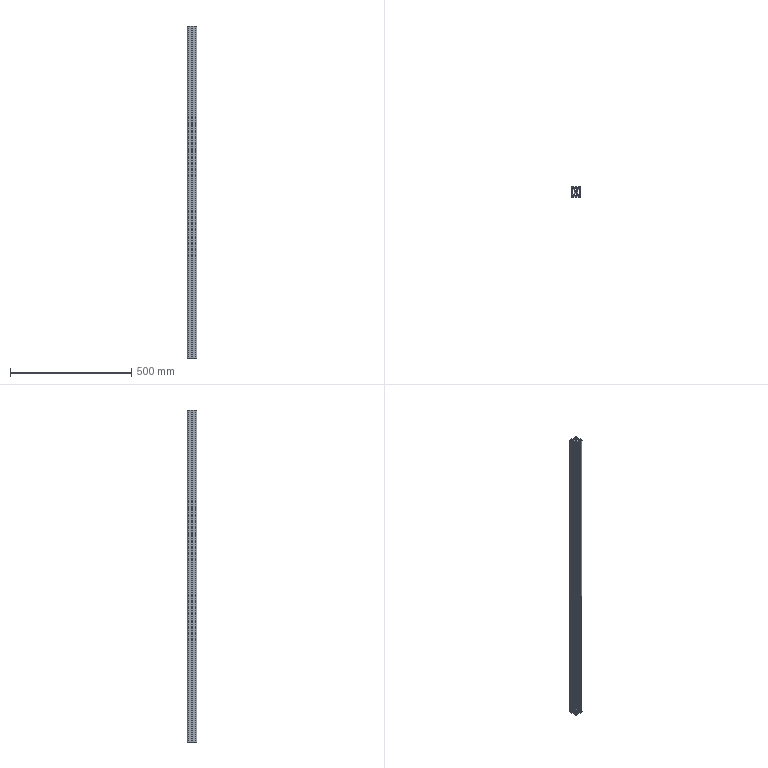Part | STEP file | 40x40-1370 | 1 solid | 88 faces | box 40 x 40 x 1370 mm | volume 964407 mm3 | plane 78 | cylinder 10 | commonest cylinder face diameters 4 x4 10 x4 6.8 x2